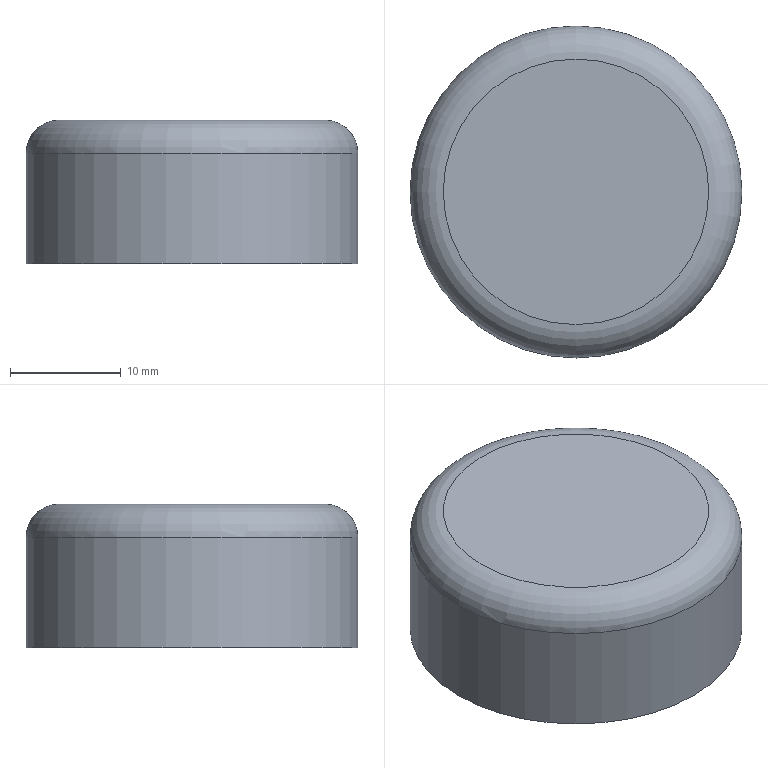Part | NX | features solid 2 | 1 solid | 4 faces | box 30 x 30 x 13 mm | volume 9015 mm3 | plane 2 | cylinder 1 | torus 1 | commonest cylinder face diameters 30 x1
STEP:
#1=CARTESIAN_POINT('',(1090.5,-131.,-360.));
#2=VERTEX_POINT('',#1);
#3=CARTESIAN_POINT('',(1075.5,-131.,-360.));
#4=DIRECTION('',(0.,0.,-1.));
#5=DIRECTION('',(1.,0.,0.));
#6=AXIS2_PLACEMENT_3D('',#3,#4,#5);
#7=CIRCLE('',#6,15.);
#8=EDGE_CURVE('',#2,#2,#7,.T.);
#9=ORIENTED_EDGE('',*,*,#8,.T.);
#10=EDGE_LOOP('',(#9));
#11=FACE_BOUND('',#10,.T.);
#12=CARTESIAN_POINT('',(1090.5,-131.,-370.));
#13=VERTEX_POINT('',#12);
#14=CARTESIAN_POINT('',(1075.5,-131.,-370.));
#15=DIRECTION('',(0.,0.,-1.));
#16=DIRECTION('',(1.,0.,0.));
#17=AXIS2_PLACEMENT_3D('',#14,#15,#16);
#18=CIRCLE('',#17,15.);
#19=EDGE_CURVE('',#13,#13,#18,.F.);
#20=ORIENTED_EDGE('',*,*,#19,.T.);
#21=EDGE_LOOP('',(#20));
#22=FACE_BOUND('',#21,.T.);
#23=CARTESIAN_POINT('',(1075.5,-131.,-360.));
#24=DIRECTION('',(0.,0.,-1.));
#25=DIRECTION('',(1.,0.,0.));
#26=AXIS2_PLACEMENT_3D('',#23,#24,#25);
#27=CYLINDRICAL_SURFACE('',#26,15.);
#28=ADVANCED_FACE('',(#11,#22),#27,.T.);
#29=CARTESIAN_POINT('',(1087.5,-131.,-357.));
#30=VERTEX_POINT('',#29);
#31=CARTESIAN_POINT('',(1075.5,-131.,-357.));
#32=DIRECTION('',(0.,0.,-1.));
#33=DIRECTION('',(1.,0.,0.));
#34=AXIS2_PLACEMENT_3D('',#31,#32,#33);
#35=CIRCLE('',#34,12.);
#36=EDGE_CURVE('',#30,#30,#35,.F.);
#37=ORIENTED_EDGE('',*,*,#36,.T.);
#38=EDGE_LOOP('',(#37));
#39=FACE_BOUND('',#38,.T.);
#40=CARTESIAN_POINT('',(1107.,-166.,-357.));
#41=DIRECTION('',(0.,0.,-1.));
#42=DIRECTION('',(1.,0.,0.));
#43=AXIS2_PLACEMENT_3D('',#40,#41,#42);
#44=PLANE('',#43);
#45=ADVANCED_FACE('',(#39),#44,.F.);
#46=ORIENTED_EDGE('',*,*,#19,.F.);
#47=EDGE_LOOP('',(#46));
#48=FACE_BOUND('',#47,.T.);
#49=CARTESIAN_POINT('',(1107.,-166.,-370.));
#50=DIRECTION('',(0.,0.,-1.));
#51=DIRECTION('',(1.,0.,0.));
#52=AXIS2_PLACEMENT_3D('',#49,#50,#51);
#53=PLANE('',#52);
#54=ADVANCED_FACE('',(#48),#53,.T.);
#55=ORIENTED_EDGE('',*,*,#8,.F.);
#56=EDGE_LOOP('',(#55));
#57=FACE_BOUND('',#56,.T.);
#58=ORIENTED_EDGE('',*,*,#36,.F.);
#59=EDGE_LOOP('',(#58));
#60=FACE_BOUND('',#59,.T.);
#61=CARTESIAN_POINT('',(1075.5,-131.,-360.));
#62=DIRECTION('',(0.,0.,-1.));
#63=DIRECTION('',(1.,0.,0.));
#64=AXIS2_PLACEMENT_3D('',#61,#62,#63);
#65=TOROIDAL_SURFACE('',#64,12.,3.);
#66=ADVANCED_FACE('',(#57,#60),#65,.T.);
#67=CLOSED_SHELL('',(#28,#45,#54,#66));
#68=MANIFOLD_SOLID_BREP('',#67);
#69=(LENGTH_UNIT()NAMED_UNIT(*)SI_UNIT(.MILLI.,.METRE.));
#70=UNCERTAINTY_MEASURE_WITH_UNIT(LENGTH_MEASURE(0.00001),#69,'','');
#71=(NAMED_UNIT(*)PLANE_ANGLE_UNIT()SI_UNIT($,.RADIAN.));
#72=(NAMED_UNIT(*)SI_UNIT($,.STERADIAN.)SOLID_ANGLE_UNIT());
#73=(GEOMETRIC_REPRESENTATION_CONTEXT(3)GLOBAL_UNCERTAINTY_ASSIGNED_CONTEXT((#70))GLOBAL_UNIT_ASSIGNED_CONTEXT((#69,#71,#72))REPRESENTATION_CONTEXT('',''));
#74=ADVANCED_BREP_SHAPE_REPRESENTATION('',(#68),#73);